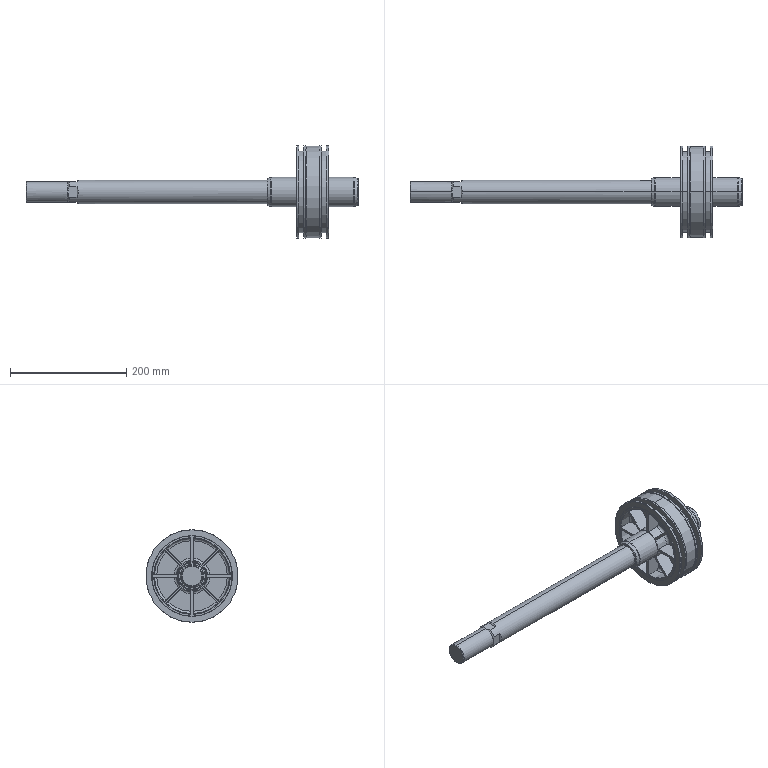Part | STEP file | 1 solid | 210 faces | box 570 x 159 x 159 mm | volume 1181996 mm3 | cone 72 | plane 70 | torus 44 | cylinder 24 | commonest cylinder face diameters 159 x8 40 x4 50 x4 140 x4 36 x2 156.9 x2